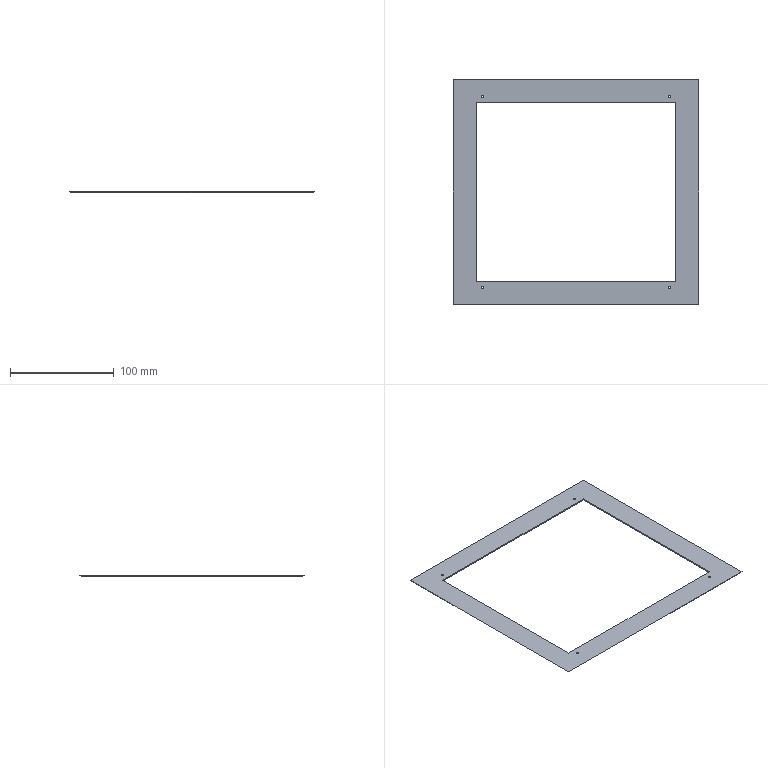Part | NX | 1 solid | 26 faces | box 236.4 x 216.4 x 1.2 mm | volume 21084 mm3 | plane 10 | cone 8 | cylinder 8 | commonest cylinder face diameters 2.5 x8
STEP:
#1=CARTESIAN_POINT('',(-117.,-107.,-75.));
#2=VERTEX_POINT('',#1);
#3=CARTESIAN_POINT('',(-117.,107.,-75.));
#4=VERTEX_POINT('',#3);
#5=CARTESIAN_POINT('',(-117.,0.,-75.));
#6=DIRECTION('',(0.,1.,0.));
#7=VECTOR('',#6,1000.);
#8=LINE('',#5,#7);
#9=EDGE_CURVE('',#2,#4,#8,.T.);
#10=ORIENTED_EDGE('',*,*,#9,.T.);
#11=CARTESIAN_POINT('',(117.,107.,-75.));
#12=VERTEX_POINT('',#11);
#13=CARTESIAN_POINT('',(0.,107.,-75.));
#14=DIRECTION('',(-1.,0.,0.));
#15=VECTOR('',#14,1000.);
#16=LINE('',#13,#15);
#17=EDGE_CURVE('',#12,#4,#16,.T.);
#18=ORIENTED_EDGE('',*,*,#17,.F.);
#19=CARTESIAN_POINT('',(117.,-107.,-75.));
#20=VERTEX_POINT('',#19);
#21=CARTESIAN_POINT('',(117.,0.,-75.));
#22=DIRECTION('',(0.,-1.,0.));
#23=VECTOR('',#22,1000.);
#24=LINE('',#21,#23);
#25=EDGE_CURVE('',#12,#20,#24,.T.);
#26=ORIENTED_EDGE('',*,*,#25,.T.);
#27=CARTESIAN_POINT('',(0.,-107.,-75.));
#28=DIRECTION('',(-1.,0.,0.));
#29=VECTOR('',#28,1000.);
#30=LINE('',#27,#29);
#31=EDGE_CURVE('',#20,#2,#30,.T.);
#32=ORIENTED_EDGE('',*,*,#31,.T.);
#33=EDGE_LOOP('',(#10,#18,#26,#32));
#34=FACE_BOUND('',#33,.T.);
#35=CARTESIAN_POINT('',(-88.3,92.,-75.));
#36=VERTEX_POINT('',#35);
#37=CARTESIAN_POINT('',(-91.7,92.,-75.));
#38=VERTEX_POINT('',#37);
#39=CARTESIAN_POINT('',(-90.,92.,-75.));
#40=DIRECTION('',(0.,0.,-1.));
#41=DIRECTION('',(-1.,0.,0.));
#42=AXIS2_PLACEMENT_3D('',#39,#40,#41);
#43=CIRCLE('',#42,1.7);
#44=EDGE_CURVE('',#36,#38,#43,.T.);
#45=ORIENTED_EDGE('',*,*,#44,.F.);
#46=CARTESIAN_POINT('',(-90.,92.,-75.));
#47=DIRECTION('',(0.,0.,-1.));
#48=DIRECTION('',(-1.,0.,0.));
#49=AXIS2_PLACEMENT_3D('',#46,#47,#48);
#50=CIRCLE('',#49,1.7);
#51=EDGE_CURVE('',#38,#36,#50,.T.);
#52=ORIENTED_EDGE('',*,*,#51,.F.);
#53=EDGE_LOOP('',(#45,#52));
#54=FACE_BOUND('',#53,.T.);
#55=CARTESIAN_POINT('',(91.7,-92.,-75.));
#56=VERTEX_POINT('',#55);
#57=CARTESIAN_POINT('',(88.3,-92.,-75.));
#58=VERTEX_POINT('',#57);
#59=CARTESIAN_POINT('',(90.,-92.,-75.));
#60=DIRECTION('',(0.,0.,-1.));
#61=DIRECTION('',(-1.,0.,0.));
#62=AXIS2_PLACEMENT_3D('',#59,#60,#61);
#63=CIRCLE('',#62,1.7);
#64=EDGE_CURVE('',#56,#58,#63,.T.);
#65=ORIENTED_EDGE('',*,*,#64,.F.);
#66=CARTESIAN_POINT('',(90.,-92.,-75.));
#67=DIRECTION('',(0.,0.,-1.));
#68=DIRECTION('',(-1.,0.,0.));
#69=AXIS2_PLACEMENT_3D('',#66,#67,#68);
#70=CIRCLE('',#69,1.7);
#71=EDGE_CURVE('',#58,#56,#70,.T.);
#72=ORIENTED_EDGE('',*,*,#71,.F.);
#73=EDGE_LOOP('',(#65,#72));
#74=FACE_BOUND('',#73,.T.);
#75=CARTESIAN_POINT('',(-88.3,-92.,-75.));
#76=VERTEX_POINT('',#75);
#77=CARTESIAN_POINT('',(-91.7,-92.,-75.));
#78=VERTEX_POINT('',#77);
#79=CARTESIAN_POINT('',(-90.,-92.,-75.));
#80=DIRECTION('',(0.,0.,-1.));
#81=DIRECTION('',(-1.,0.,0.));
#82=AXIS2_PLACEMENT_3D('',#79,#80,#81);
#83=CIRCLE('',#82,1.7);
#84=EDGE_CURVE('',#76,#78,#83,.T.);
#85=ORIENTED_EDGE('',*,*,#84,.F.);
#86=CARTESIAN_POINT('',(-90.,-92.,-75.));
#87=DIRECTION('',(0.,0.,-1.));
#88=DIRECTION('',(-1.,0.,0.));
#89=AXIS2_PLACEMENT_3D('',#86,#87,#88);
#90=CIRCLE('',#89,1.7);
#91=EDGE_CURVE('',#78,#76,#90,.T.);
#92=ORIENTED_EDGE('',*,*,#91,.F.);
#93=EDGE_LOOP('',(#85,#92));
#94=FACE_BOUND('',#93,.T.);
#95=CARTESIAN_POINT('',(91.7,92.,-75.));
#96=VERTEX_POINT('',#95);
#97=CARTESIAN_POINT('',(88.3,92.,-75.));
#98=VERTEX_POINT('',#97);
#99=CARTESIAN_POINT('',(90.,92.,-75.));
#100=DIRECTION('',(0.,0.,-1.));
#101=DIRECTION('',(-1.,0.,0.));
#102=AXIS2_PLACEMENT_3D('',#99,#100,#101);
#103=CIRCLE('',#102,1.7);
#104=EDGE_CURVE('',#96,#98,#103,.T.);
#105=ORIENTED_EDGE('',*,*,#104,.F.);
#106=CARTESIAN_POINT('',(90.,92.,-75.));
#107=DIRECTION('',(0.,0.,-1.));
#108=DIRECTION('',(-1.,0.,0.));
#109=AXIS2_PLACEMENT_3D('',#106,#107,#108);
#110=CIRCLE('',#109,1.7);
#111=EDGE_CURVE('',#98,#96,#110,.T.);
#112=ORIENTED_EDGE('',*,*,#111,.F.);
#113=EDGE_LOOP('',(#105,#112));
#114=FACE_BOUND('',#113,.T.);
#115=CARTESIAN_POINT('',(-96.,86.,-75.));
#116=VERTEX_POINT('',#115);
#117=CARTESIAN_POINT('',(96.,86.,-75.));
#118=VERTEX_POINT('',#117);
#119=CARTESIAN_POINT('',(0.,86.,-75.));
#120=DIRECTION('',(1.,0.,0.));
#121=VECTOR('',#120,1000.);
#122=LINE('',#119,#121);
#123=EDGE_CURVE('',#116,#118,#122,.T.);
#124=ORIENTED_EDGE('',*,*,#123,.F.);
#125=CARTESIAN_POINT('',(-96.,-86.,-75.));
#126=VERTEX_POINT('',#125);
#127=CARTESIAN_POINT('',(-96.,0.,-75.));
#128=DIRECTION('',(0.,1.,0.));
#129=VECTOR('',#128,1000.);
#130=LINE('',#127,#129);
#131=EDGE_CURVE('',#126,#116,#130,.T.);
#132=ORIENTED_EDGE('',*,*,#131,.F.);
#133=CARTESIAN_POINT('',(96.,-86.,-75.));
#134=VERTEX_POINT('',#133);
#135=CARTESIAN_POINT('',(0.,-86.,-75.));
#136=DIRECTION('',(-1.,0.,0.));
#137=VECTOR('',#136,1000.);
#138=LINE('',#135,#137);
#139=EDGE_CURVE('',#134,#126,#138,.T.);
#140=ORIENTED_EDGE('',*,*,#139,.F.);
#141=CARTESIAN_POINT('',(96.,0.,-75.));
#142=DIRECTION('',(0.,-1.,0.));
#143=VECTOR('',#142,1000.);
#144=LINE('',#141,#143);
#145=EDGE_CURVE('',#118,#134,#144,.T.);
#146=ORIENTED_EDGE('',*,*,#145,.F.);
#147=EDGE_LOOP('',(#124,#132,#140,#146));
#148=FACE_BOUND('',#147,.T.);
#149=CARTESIAN_POINT('',(0.,0.,-75.));
#150=DIRECTION('',(0.,0.,1.));
#151=DIRECTION('',(1.,0.,0.));
#152=AXIS2_PLACEMENT_3D('',#149,#150,#151);
#153=PLANE('',#152);
#154=ADVANCED_FACE('',(#34,#54,#74,#94,#114,#148),#153,.F.);
#155=CARTESIAN_POINT('',(-88.75,92.,-74.74));
#156=VERTEX_POINT('',#155);
#157=CARTESIAN_POINT('',(-91.25,92.,-74.74));
#158=VERTEX_POINT('',#157);
#159=CARTESIAN_POINT('',(-90.,92.,-74.74));
#160=DIRECTION('',(0.,0.,-1.));
#161=DIRECTION('',(-1.,0.,0.));
#162=AXIS2_PLACEMENT_3D('',#159,#160,#161);
#163=CIRCLE('',#162,1.25);
#164=EDGE_CURVE('',#156,#158,#163,.T.);
#165=ORIENTED_EDGE('',*,*,#164,.F.);
#166=CARTESIAN_POINT('',(-88.75,92.,-74.74));
#167=DIRECTION('',(0.866,0.,-0.5));
#168=VECTOR('',#167,1000.);
#169=LINE('',#166,#168);
#170=EDGE_CURVE('',#36,#156,#169,.F.);
#171=ORIENTED_EDGE('',*,*,#170,.F.);
#172=ORIENTED_EDGE('',*,*,#44,.T.);
#173=CARTESIAN_POINT('',(-91.25,92.,-74.74));
#174=DIRECTION('',(-0.866,0.,-0.5));
#175=VECTOR('',#174,1000.);
#176=LINE('',#173,#175);
#177=EDGE_CURVE('',#38,#158,#176,.F.);
#178=ORIENTED_EDGE('',*,*,#177,.T.);
#179=EDGE_LOOP('',(#165,#171,#172,#178));
#180=FACE_BOUND('',#179,.T.);
#181=CARTESIAN_POINT('',(-90.,92.,-74.74));
#182=DIRECTION('',(0.,0.,-1.));
#183=DIRECTION('',(-1.,0.,0.));
#184=AXIS2_PLACEMENT_3D('',#181,#182,#183);
#185=CONICAL_SURFACE('',#184,1.25,1.047);
#186=ADVANCED_FACE('',(#180),#185,.F.);
#187=ORIENTED_EDGE('',*,*,#164,.T.);
#188=CARTESIAN_POINT('',(-91.25,92.,-73.8));
#189=VERTEX_POINT('',#188);
#190=CARTESIAN_POINT('',(-91.25,92.,-75.));
#191=DIRECTION('',(0.,0.,-1.));
#192=VECTOR('',#191,1000.);
#193=LINE('',#190,#192);
#194=EDGE_CURVE('',#158,#189,#193,.F.);
#195=ORIENTED_EDGE('',*,*,#194,.T.);
#196=CARTESIAN_POINT('',(-88.75,92.,-73.8));
#197=VERTEX_POINT('',#196);
#198=CARTESIAN_POINT('',(-90.,92.,-73.8));
#199=DIRECTION('',(0.,0.,-1.));
#200=DIRECTION('',(-1.,0.,0.));
#201=AXIS2_PLACEMENT_3D('',#198,#199,#200);
#202=CIRCLE('',#201,1.25);
#203=EDGE_CURVE('',#197,#189,#202,.T.);
#204=ORIENTED_EDGE('',*,*,#203,.F.);
#205=CARTESIAN_POINT('',(-88.75,92.,-75.));
#206=DIRECTION('',(0.,0.,-1.));
#207=VECTOR('',#206,1000.);
#208=LINE('',#205,#207);
#209=EDGE_CURVE('',#156,#197,#208,.F.);
#210=ORIENTED_EDGE('',*,*,#209,.F.);
#211=EDGE_LOOP('',(#187,#195,#204,#210));
#212=FACE_BOUND('',#211,.T.);
#213=CARTESIAN_POINT('',(-90.,92.,-75.));
#214=DIRECTION('',(0.,0.,-1.));
#215=DIRECTION('',(-1.,0.,0.));
#216=AXIS2_PLACEMENT_3D('',#213,#214,#215);
#217=CYLINDRICAL_SURFACE('',#216,1.25);
#218=ADVANCED_FACE('',(#212),#217,.F.);
#219=CARTESIAN_POINT('',(118.2,108.2,-73.8));
#220=VERTEX_POINT('',#219);
#221=CARTESIAN_POINT('',(118.2,-108.2,-73.8));
#222=VERTEX_POINT('',#221);
#223=CARTESIAN_POINT('',(118.2,0.,-73.8));
#224=DIRECTION('',(0.,-1.,0.));
#225=VECTOR('',#224,1000.);
#226=LINE('',#223,#225);
#227=EDGE_CURVE('',#220,#222,#226,.T.);
#228=ORIENTED_EDGE('',*,*,#227,.F.);
#229=CARTESIAN_POINT('',(-118.2,108.2,-73.8));
#230=VERTEX_POINT('',#229);
#231=CARTESIAN_POINT('',(0.,108.2,-73.8));
#232=DIRECTION('',(1.,0.,0.));
#233=VECTOR('',#232,1000.);
#234=LINE('',#231,#233);
#235=EDGE_CURVE('',#230,#220,#234,.T.);
#236=ORIENTED_EDGE('',*,*,#235,.F.);
#237=CARTESIAN_POINT('',(-118.2,-108.2,-73.8));
#238=VERTEX_POINT('',#237);
#239=CARTESIAN_POINT('',(-118.2,0.,-73.8));
#240=DIRECTION('',(0.,1.,0.));
#241=VECTOR('',#240,1000.);
#242=LINE('',#239,#241);
#243=EDGE_CURVE('',#238,#230,#242,.T.);
#244=ORIENTED_EDGE('',*,*,#243,.F.);
#245=CARTESIAN_POINT('',(0.,-108.2,-73.8));
#246=DIRECTION('',(1.,0.,0.));
#247=VECTOR('',#246,1000.);
#248=LINE('',#245,#247);
#249=EDGE_CURVE('',#238,#222,#248,.T.);
#250=ORIENTED_EDGE('',*,*,#249,.T.);
#251=EDGE_LOOP('',(#228,#236,#244,#250));
#252=FACE_BOUND('',#251,.T.);
#253=CARTESIAN_POINT('',(96.,86.,-73.8));
#254=VERTEX_POINT('',#253);
#255=CARTESIAN_POINT('',(-96.,86.,-73.8));
#256=VERTEX_POINT('',#255);
#257=CARTESIAN_POINT('',(0.,86.,-73.8));
#258=DIRECTION('',(-1.,0.,0.));
#259=VECTOR('',#258,1000.);
#260=LINE('',#257,#259);
#261=EDGE_CURVE('',#254,#256,#260,.T.);
#262=ORIENTED_EDGE('',*,*,#261,.F.);
#263=CARTESIAN_POINT('',(96.,-86.,-73.8));
#264=VERTEX_POINT('',#263);
#265=CARTESIAN_POINT('',(96.,0.,-73.8));
#266=DIRECTION('',(0.,1.,0.));
#267=VECTOR('',#266,1000.);
#268=LINE('',#265,#267);
#269=EDGE_CURVE('',#264,#254,#268,.T.);
#270=ORIENTED_EDGE('',*,*,#269,.F.);
#271=CARTESIAN_POINT('',(-96.,-86.,-73.8));
#272=VERTEX_POINT('',#271);
#273=CARTESIAN_POINT('',(0.,-86.,-73.8));
#274=DIRECTION('',(1.,0.,0.));
#275=VECTOR('',#274,1000.);
#276=LINE('',#273,#275);
#277=EDGE_CURVE('',#272,#264,#276,.T.);
#278=ORIENTED_EDGE('',*,*,#277,.F.);
#279=CARTESIAN_POINT('',(-96.,0.,-73.8));
#280=DIRECTION('',(0.,-1.,0.));
#281=VECTOR('',#280,1000.);
#282=LINE('',#279,#281);
#283=EDGE_CURVE('',#256,#272,#282,.T.);
#284=ORIENTED_EDGE('',*,*,#283,.F.);
#285=EDGE_LOOP('',(#262,#270,#278,#284));
#286=FACE_BOUND('',#285,.T.);
#287=CARTESIAN_POINT('',(-88.75,-92.,-73.8));
#288=VERTEX_POINT('',#287);
#289=CARTESIAN_POINT('',(-91.25,-92.,-73.8));
#290=VERTEX_POINT('',#289);
#291=CARTESIAN_POINT('',(-90.,-92.,-73.8));
#292=DIRECTION('',(0.,0.,-1.));
#293=DIRECTION('',(-1.,0.,0.));
#294=AXIS2_PLACEMENT_3D('',#291,#292,#293);
#295=CIRCLE('',#294,1.25);
#296=EDGE_CURVE('',#288,#290,#295,.T.);
#297=ORIENTED_EDGE('',*,*,#296,.T.);
#298=CARTESIAN_POINT('',(-90.,-92.,-73.8));
#299=DIRECTION('',(0.,0.,-1.));
#300=DIRECTION('',(-1.,0.,0.));
#301=AXIS2_PLACEMENT_3D('',#298,#299,#300);
#302=CIRCLE('',#301,1.25);
#303=EDGE_CURVE('',#290,#288,#302,.T.);
#304=ORIENTED_EDGE('',*,*,#303,.T.);
#305=EDGE_LOOP('',(#297,#304));
#306=FACE_BOUND('',#305,.T.);
#307=CARTESIAN_POINT('',(91.25,-92.,-73.8));
#308=VERTEX_POINT('',#307);
#309=CARTESIAN_POINT('',(88.75,-92.,-73.8));
#310=VERTEX_POINT('',#309);
#311=CARTESIAN_POINT('',(90.,-92.,-73.8));
#312=DIRECTION('',(0.,0.,-1.));
#313=DIRECTION('',(-1.,0.,0.));
#314=AXIS2_PLACEMENT_3D('',#311,#312,#313);
#315=CIRCLE('',#314,1.25);
#316=EDGE_CURVE('',#308,#310,#315,.T.);
#317=ORIENTED_EDGE('',*,*,#316,.T.);
#318=CARTESIAN_POINT('',(90.,-92.,-73.8));
#319=DIRECTION('',(0.,0.,-1.));
#320=DIRECTION('',(-1.,0.,0.));
#321=AXIS2_PLACEMENT_3D('',#318,#319,#320);
#322=CIRCLE('',#321,1.25);
#323=EDGE_CURVE('',#310,#308,#322,.T.);
#324=ORIENTED_EDGE('',*,*,#323,.T.);
#325=EDGE_LOOP('',(#317,#324));
#326=FACE_BOUND('',#325,.T.);
#327=CARTESIAN_POINT('',(91.25,92.,-73.8));
#328=VERTEX_POINT('',#327);
#329=CARTESIAN_POINT('',(88.75,92.,-73.8));
#330=VERTEX_POINT('',#329);
#331=CARTESIAN_POINT('',(90.,92.,-73.8));
#332=DIRECTION('',(0.,0.,-1.));
#333=DIRECTION('',(-1.,0.,0.));
#334=AXIS2_PLACEMENT_3D('',#331,#332,#333);
#335=CIRCLE('',#334,1.25);
#336=EDGE_CURVE('',#328,#330,#335,.T.);
#337=ORIENTED_EDGE('',*,*,#336,.T.);
#338=CARTESIAN_POINT('',(90.,92.,-73.8));
#339=DIRECTION('',(0.,0.,-1.));
#340=DIRECTION('',(-1.,0.,0.));
#341=AXIS2_PLACEMENT_3D('',#338,#339,#340);
#342=CIRCLE('',#341,1.25);
#343=EDGE_CURVE('',#330,#328,#342,.T.);
#344=ORIENTED_EDGE('',*,*,#343,.T.);
#345=EDGE_LOOP('',(#337,#344));
#346=FACE_BOUND('',#345,.T.);
#347=ORIENTED_EDGE('',*,*,#203,.T.);
#348=CARTESIAN_POINT('',(-90.,92.,-73.8));
#349=DIRECTION('',(0.,0.,-1.));
#350=DIRECTION('',(-1.,0.,0.));
#351=AXIS2_PLACEMENT_3D('',#348,#349,#350);
#352=CIRCLE('',#351,1.25);
#353=EDGE_CURVE('',#189,#197,#352,.T.);
#354=ORIENTED_EDGE('',*,*,#353,.T.);
#355=EDGE_LOOP('',(#347,#354));
#356=FACE_BOUND('',#355,.T.);
#357=CARTESIAN_POINT('',(0.,0.,-73.8));
#358=DIRECTION('',(0.,0.,-1.));
#359=DIRECTION('',(0.,-1.,0.));
#360=AXIS2_PLACEMENT_3D('',#357,#358,#359);
#361=PLANE('',#360);
#362=ADVANCED_FACE('',(#252,#286,#306,#326,#346,#356),#361,.F.);
#363=ORIENTED_EDGE('',*,*,#9,.F.);
#364=CARTESIAN_POINT('',(-192.,-182.,0.));
#365=DIRECTION('',(0.5774,0.5774,-0.5774));
#366=VECTOR('',#365,1000.);
#367=LINE('',#364,#366);
#368=EDGE_CURVE('',#238,#2,#367,.T.);
#369=ORIENTED_EDGE('',*,*,#368,.F.);
#370=ORIENTED_EDGE('',*,*,#243,.T.);
#371=CARTESIAN_POINT('',(-192.,182.,0.));
#372=DIRECTION('',(0.5774,-0.5774,-0.5774));
#373=VECTOR('',#372,1000.);
#374=LINE('',#371,#373);
#375=EDGE_CURVE('',#230,#4,#374,.T.);
#376=ORIENTED_EDGE('',*,*,#375,.T.);
#377=EDGE_LOOP('',(#363,#369,#370,#376));
#378=FACE_BOUND('',#377,.T.);
#379=CARTESIAN_POINT('',(-118.5,0.,-73.5));
#380=DIRECTION('',(-0.7071,0.,-0.7071));
#381=DIRECTION('',(-0.7071,0.,0.7071));
#382=AXIS2_PLACEMENT_3D('',#379,#380,#381);
#383=PLANE('',#382);
#384=ADVANCED_FACE('',(#378),#383,.T.);
#385=ORIENTED_EDGE('',*,*,#25,.F.);
#386=CARTESIAN_POINT('',(192.,182.,0.));
#387=DIRECTION('',(-0.5774,-0.5774,-0.5774));
#388=VECTOR('',#387,1000.);
#389=LINE('',#386,#388);
#390=EDGE_CURVE('',#220,#12,#389,.T.);
#391=ORIENTED_EDGE('',*,*,#390,.F.);
#392=ORIENTED_EDGE('',*,*,#227,.T.);
#393=CARTESIAN_POINT('',(192.,-182.,0.));
#394=DIRECTION('',(-0.5774,0.5774,-0.5774));
#395=VECTOR('',#394,1000.);
#396=LINE('',#393,#395);
#397=EDGE_CURVE('',#222,#20,#396,.T.);
#398=ORIENTED_EDGE('',*,*,#397,.T.);
#399=EDGE_LOOP('',(#385,#391,#392,#398));
#400=FACE_BOUND('',#399,.T.);
#401=CARTESIAN_POINT('',(118.5,0.,-73.5));
#402=DIRECTION('',(0.7071,0.,-0.7071));
#403=DIRECTION('',(0.,-1.,0.));
#404=AXIS2_PLACEMENT_3D('',#401,#402,#403);
#405=PLANE('',#404);
#406=ADVANCED_FACE('',(#400),#405,.T.);
#407=ORIENTED_EDGE('',*,*,#235,.T.);
#408=ORIENTED_EDGE('',*,*,#390,.T.);
#409=ORIENTED_EDGE('',*,*,#17,.T.);
#410=ORIENTED_EDGE('',*,*,#375,.F.);
#411=EDGE_LOOP('',(#407,#408,#409,#410));
#412=FACE_BOUND('',#411,.T.);
#413=CARTESIAN_POINT('',(0.,108.5,-73.5));
#414=DIRECTION('',(0.,0.7071,-0.7071));
#415=DIRECTION('',(-1.,0.,0.));
#416=AXIS2_PLACEMENT_3D('',#413,#414,#415);
#417=PLANE('',#416);
#418=ADVANCED_FACE('',(#412),#417,.T.);
#419=ORIENTED_EDGE('',*,*,#249,.F.);
#420=ORIENTED_EDGE('',*,*,#368,.T.);
#421=ORIENTED_EDGE('',*,*,#31,.F.);
#422=ORIENTED_EDGE('',*,*,#397,.F.);
#423=EDGE_LOOP('',(#419,#420,#421,#422));
#424=FACE_BOUND('',#423,.T.);
#425=CARTESIAN_POINT('',(0.,-108.5,-73.5));
#426=DIRECTION('',(0.,0.7071,0.7071));
#427=DIRECTION('',(1.,0.,0.));
#428=AXIS2_PLACEMENT_3D('',#425,#426,#427);
#429=PLANE('',#428);
#430=ADVANCED_FACE('',(#424),#429,.F.);
#431=ORIENTED_EDGE('',*,*,#261,.T.);
#432=CARTESIAN_POINT('',(-96.,86.,-73.8));
#433=DIRECTION('',(0.,0.,-1.));
#434=VECTOR('',#433,1000.);
#435=LINE('',#432,#434);
#436=EDGE_CURVE('',#256,#116,#435,.T.);
#437=ORIENTED_EDGE('',*,*,#436,.T.);
#438=ORIENTED_EDGE('',*,*,#123,.T.);
#439=CARTESIAN_POINT('',(96.,86.,-73.8));
#440=DIRECTION('',(0.,0.,-1.));
#441=VECTOR('',#440,1000.);
#442=LINE('',#439,#441);
#443=EDGE_CURVE('',#254,#118,#442,.T.);
#444=ORIENTED_EDGE('',*,*,#443,.F.);
#445=EDGE_LOOP('',(#431,#437,#438,#444));
#446=FACE_BOUND('',#445,.T.);
#447=CARTESIAN_POINT('',(-96.,86.,-75.));
#448=DIRECTION('',(0.,1.,0.));
#449=DIRECTION('',(1.,0.,0.));
#450=AXIS2_PLACEMENT_3D('',#447,#448,#449);
#451=PLANE('',#450);
#452=ADVANCED_FACE('',(#446),#451,.F.);
#453=ORIENTED_EDGE('',*,*,#277,.T.);
#454=CARTESIAN_POINT('',(96.,-86.,-73.8));
#455=DIRECTION('',(0.,0.,-1.));
#456=VECTOR('',#455,1000.);
#457=LINE('',#454,#456);
#458=EDGE_CURVE('',#264,#134,#457,.T.);
#459=ORIENTED_EDGE('',*,*,#458,.T.);
#460=ORIENTED_EDGE('',*,*,#139,.T.);
#461=CARTESIAN_POINT('',(-96.,-86.,-73.8));
#462=DIRECTION('',(0.,0.,-1.));
#463=VECTOR('',#462,1000.);
#464=LINE('',#461,#463);
#465=EDGE_CURVE('',#272,#126,#464,.T.);
#466=ORIENTED_EDGE('',*,*,#465,.F.);
#467=EDGE_LOOP('',(#453,#459,#460,#466));
#468=FACE_BOUND('',#467,.T.);
#469=CARTESIAN_POINT('',(96.,-86.,-75.));
#470=DIRECTION('',(0.,-1.,0.));
#471=DIRECTION('',(0.,0.,-1.));
#472=AXIS2_PLACEMENT_3D('',#469,#470,#471);
#473=PLANE('',#472);
#474=ADVANCED_FACE('',(#468),#473,.F.);
#475=ORIENTED_EDGE('',*,*,#283,.T.);
#476=ORIENTED_EDGE('',*,*,#465,.T.);
#477=ORIENTED_EDGE('',*,*,#131,.T.);
#478=ORIENTED_EDGE('',*,*,#436,.F.);
#479=EDGE_LOOP('',(#475,#476,#477,#478));
#480=FACE_BOUND('',#479,.T.);
#481=CARTESIAN_POINT('',(-96.,-86.,-75.));
#482=DIRECTION('',(-1.,0.,0.));
#483=DIRECTION('',(0.,0.,1.));
#484=AXIS2_PLACEMENT_3D('',#481,#482,#483);
#485=PLANE('',#484);
#486=ADVANCED_FACE('',(#480),#485,.F.);
#487=ORIENTED_EDGE('',*,*,#269,.T.);
#488=ORIENTED_EDGE('',*,*,#443,.T.);
#489=ORIENTED_EDGE('',*,*,#145,.T.);
#490=ORIENTED_EDGE('',*,*,#458,.F.);
#491=EDGE_LOOP('',(#487,#488,#489,#490));
#492=FACE_BOUND('',#491,.T.);
#493=CARTESIAN_POINT('',(96.,86.,-75.));
#494=DIRECTION('',(1.,0.,0.));
#495=DIRECTION('',(0.,1.,0.));
#496=AXIS2_PLACEMENT_3D('',#493,#494,#495);
#497=PLANE('',#496);
#498=ADVANCED_FACE('',(#492),#497,.F.);
#499=CARTESIAN_POINT('',(-88.75,-92.,-74.74));
#500=VERTEX_POINT('',#499);
#501=CARTESIAN_POINT('',(-91.25,-92.,-74.74));
#502=VERTEX_POINT('',#501);
#503=CARTESIAN_POINT('',(-90.,-92.,-74.74));
#504=DIRECTION('',(0.,0.,-1.));
#505=DIRECTION('',(-1.,0.,0.));
#506=AXIS2_PLACEMENT_3D('',#503,#504,#505);
#507=CIRCLE('',#506,1.25);
#508=EDGE_CURVE('',#500,#502,#507,.T.);
#509=ORIENTED_EDGE('',*,*,#508,.T.);
#510=CARTESIAN_POINT('',(-91.25,-92.,-75.));
#511=DIRECTION('',(0.,0.,-1.));
#512=VECTOR('',#511,1000.);
#513=LINE('',#510,#512);
#514=EDGE_CURVE('',#502,#290,#513,.F.);
#515=ORIENTED_EDGE('',*,*,#514,.T.);
#516=ORIENTED_EDGE('',*,*,#296,.F.);
#517=CARTESIAN_POINT('',(-88.75,-92.,-75.));
#518=DIRECTION('',(0.,0.,-1.));
#519=VECTOR('',#518,1000.);
#520=LINE('',#517,#519);
#521=EDGE_CURVE('',#500,#288,#520,.F.);
#522=ORIENTED_EDGE('',*,*,#521,.F.);
#523=EDGE_LOOP('',(#509,#515,#516,#522));
#524=FACE_BOUND('',#523,.T.);
#525=CARTESIAN_POINT('',(-90.,-92.,-75.));
#526=DIRECTION('',(0.,0.,-1.));
#527=DIRECTION('',(-1.,0.,0.));
#528=AXIS2_PLACEMENT_3D('',#525,#526,#527);
#529=CYLINDRICAL_SURFACE('',#528,1.25);
#530=ADVANCED_FACE('',(#524),#529,.F.);
#531=ORIENTED_EDGE('',*,*,#508,.F.);
#532=CARTESIAN_POINT('',(-88.75,-92.,-74.74));
#533=DIRECTION('',(0.866,0.,-0.5));
#534=VECTOR('',#533,1000.);
#535=LINE('',#532,#534);
#536=EDGE_CURVE('',#76,#500,#535,.F.);
#537=ORIENTED_EDGE('',*,*,#536,.F.);
#538=ORIENTED_EDGE('',*,*,#84,.T.);
#539=CARTESIAN_POINT('',(-91.25,-92.,-74.74));
#540=DIRECTION('',(-0.866,0.,-0.5));
#541=VECTOR('',#540,1000.);
#542=LINE('',#539,#541);
#543=EDGE_CURVE('',#78,#502,#542,.F.);
#544=ORIENTED_EDGE('',*,*,#543,.T.);
#545=EDGE_LOOP('',(#531,#537,#538,#544));
#546=FACE_BOUND('',#545,.T.);
#547=CARTESIAN_POINT('',(-90.,-92.,-74.74));
#548=DIRECTION('',(0.,0.,-1.));
#549=DIRECTION('',(-1.,0.,0.));
#550=AXIS2_PLACEMENT_3D('',#547,#548,#549);
#551=CONICAL_SURFACE('',#550,1.25,1.047);
#552=ADVANCED_FACE('',(#546),#551,.F.);
#553=CARTESIAN_POINT('',(91.25,-92.,-74.74));
#554=VERTEX_POINT('',#553);
#555=CARTESIAN_POINT('',(88.75,-92.,-74.74));
#556=VERTEX_POINT('',#555);
#557=CARTESIAN_POINT('',(90.,-92.,-74.74));
#558=DIRECTION('',(0.,0.,-1.));
#559=DIRECTION('',(-1.,0.,0.));
#560=AXIS2_PLACEMENT_3D('',#557,#558,#559);
#561=CIRCLE('',#560,1.25);
#562=EDGE_CURVE('',#554,#556,#561,.T.);
#563=ORIENTED_EDGE('',*,*,#562,.T.);
#564=CARTESIAN_POINT('',(88.75,-92.,-75.));
#565=DIRECTION('',(0.,0.,-1.));
#566=VECTOR('',#565,1000.);
#567=LINE('',#564,#566);
#568=EDGE_CURVE('',#556,#310,#567,.F.);
#569=ORIENTED_EDGE('',*,*,#568,.T.);
#570=ORIENTED_EDGE('',*,*,#316,.F.);
#571=CARTESIAN_POINT('',(91.25,-92.,-75.));
#572=DIRECTION('',(0.,0.,-1.));
#573=VECTOR('',#572,1000.);
#574=LINE('',#571,#573);
#575=EDGE_CURVE('',#554,#308,#574,.F.);
#576=ORIENTED_EDGE('',*,*,#575,.F.);
#577=EDGE_LOOP('',(#563,#569,#570,#576));
#578=FACE_BOUND('',#577,.T.);
#579=CARTESIAN_POINT('',(90.,-92.,-75.));
#580=DIRECTION('',(0.,0.,-1.));
#581=DIRECTION('',(-1.,0.,0.));
#582=AXIS2_PLACEMENT_3D('',#579,#580,#581);
#583=CYLINDRICAL_SURFACE('',#582,1.25);
#584=ADVANCED_FACE('',(#578),#583,.F.);
#585=ORIENTED_EDGE('',*,*,#562,.F.);
#586=CARTESIAN_POINT('',(91.25,-92.,-74.74));
#587=DIRECTION('',(0.866,0.,-0.5));
#588=VECTOR('',#587,1000.);
#589=LINE('',#586,#588);
#590=EDGE_CURVE('',#56,#554,#589,.F.);
#591=ORIENTED_EDGE('',*,*,#590,.F.);
#592=ORIENTED_EDGE('',*,*,#64,.T.);
#593=CARTESIAN_POINT('',(88.75,-92.,-74.74));
#594=DIRECTION('',(-0.866,0.,-0.5));
#595=VECTOR('',#594,1000.);
#596=LINE('',#593,#595);
#597=EDGE_CURVE('',#58,#556,#596,.F.);
#598=ORIENTED_EDGE('',*,*,#597,.T.);
#599=EDGE_LOOP('',(#585,#591,#592,#598));
#600=FACE_BOUND('',#599,.T.);
#601=CARTESIAN_POINT('',(90.,-92.,-74.74));
#602=DIRECTION('',(0.,0.,-1.));
#603=DIRECTION('',(-1.,0.,0.));
#604=AXIS2_PLACEMENT_3D('',#601,#602,#603);
#605=CONICAL_SURFACE('',#604,1.25,1.047);
#606=ADVANCED_FACE('',(#600),#605,.F.);
#607=CARTESIAN_POINT('',(91.25,92.,-74.74));
#608=VERTEX_POINT('',#607);
#609=CARTESIAN_POINT('',(88.75,92.,-74.74));
#610=VERTEX_POINT('',#609);
#611=CARTESIAN_POINT('',(90.,92.,-74.74));
#612=DIRECTION('',(0.,0.,-1.));
#613=DIRECTION('',(-1.,0.,0.));
#614=AXIS2_PLACEMENT_3D('',#611,#612,#613);
#615=CIRCLE('',#614,1.25);
#616=EDGE_CURVE('',#608,#610,#615,.T.);
#617=ORIENTED_EDGE('',*,*,#616,.T.);
#618=CARTESIAN_POINT('',(88.75,92.,-75.));
#619=DIRECTION('',(0.,0.,-1.));
#620=VECTOR('',#619,1000.);
#621=LINE('',#618,#620);
#622=EDGE_CURVE('',#610,#330,#621,.F.);
#623=ORIENTED_EDGE('',*,*,#622,.T.);
#624=ORIENTED_EDGE('',*,*,#336,.F.);
#625=CARTESIAN_POINT('',(91.25,92.,-75.));
#626=DIRECTION('',(0.,0.,-1.));
#627=VECTOR('',#626,1000.);
#628=LINE('',#625,#627);
#629=EDGE_CURVE('',#608,#328,#628,.F.);
#630=ORIENTED_EDGE('',*,*,#629,.F.);
#631=EDGE_LOOP('',(#617,#623,#624,#630));
#632=FACE_BOUND('',#631,.T.);
#633=CARTESIAN_POINT('',(90.,92.,-75.));
#634=DIRECTION('',(0.,0.,-1.));
#635=DIRECTION('',(-1.,0.,0.));
#636=AXIS2_PLACEMENT_3D('',#633,#634,#635);
#637=CYLINDRICAL_SURFACE('',#636,1.25);
#638=ADVANCED_FACE('',(#632),#637,.F.);
#639=ORIENTED_EDGE('',*,*,#616,.F.);
#640=CARTESIAN_POINT('',(91.25,92.,-74.74));
#641=DIRECTION('',(0.866,0.,-0.5));
#642=VECTOR('',#641,1000.);
#643=LINE('',#640,#642);
#644=EDGE_CURVE('',#96,#608,#643,.F.);
#645=ORIENTED_EDGE('',*,*,#644,.F.);
#646=ORIENTED_EDGE('',*,*,#104,.T.);
#647=CARTESIAN_POINT('',(88.75,92.,-74.74));
#648=DIRECTION('',(-0.866,0.,-0.5));
#649=VECTOR('',#648,1000.);
#650=LINE('',#647,#649);
#651=EDGE_CURVE('',#98,#610,#650,.F.);
#652=ORIENTED_EDGE('',*,*,#651,.T.);
#653=EDGE_LOOP('',(#639,#645,#646,#652));
#654=FACE_BOUND('',#653,.T.);
#655=CARTESIAN_POINT('',(90.,92.,-74.74));
#656=DIRECTION('',(0.,0.,-1.));
#657=DIRECTION('',(-1.,0.,0.));
#658=AXIS2_PLACEMENT_3D('',#655,#656,#657);
#659=CONICAL_SURFACE('',#658,1.25,1.047);
#660=ADVANCED_FACE('',(#654),#659,.F.);
#661=ORIENTED_EDGE('',*,*,#568,.F.);
#662=CARTESIAN_POINT('',(90.,-92.,-74.74));
#663=DIRECTION('',(0.,0.,-1.));
#664=DIRECTION('',(-1.,0.,0.));
#665=AXIS2_PLACEMENT_3D('',#662,#663,#664);
#666=CIRCLE('',#665,1.25);
#667=EDGE_CURVE('',#556,#554,#666,.T.);
#668=ORIENTED_EDGE('',*,*,#667,.T.);
#669=ORIENTED_EDGE('',*,*,#575,.T.);
#670=ORIENTED_EDGE('',*,*,#323,.F.);
#671=EDGE_LOOP('',(#661,#668,#669,#670));
#672=FACE_BOUND('',#671,.T.);
#673=CARTESIAN_POINT('',(90.,-92.,-75.));
#674=DIRECTION('',(0.,0.,-1.));
#675=DIRECTION('',(-1.,0.,0.));
#676=AXIS2_PLACEMENT_3D('',#673,#674,#675);
#677=CYLINDRICAL_SURFACE('',#676,1.25);
#678=ADVANCED_FACE('',(#672),#677,.F.);
#679=ORIENTED_EDGE('',*,*,#597,.F.);
#680=ORIENTED_EDGE('',*,*,#71,.T.);
#681=ORIENTED_EDGE('',*,*,#590,.T.);
#682=ORIENTED_EDGE('',*,*,#667,.F.);
#683=EDGE_LOOP('',(#679,#680,#681,#682));
#684=FACE_BOUND('',#683,.T.);
#685=CARTESIAN_POINT('',(90.,-92.,-74.74));
#686=DIRECTION('',(0.,0.,-1.));
#687=DIRECTION('',(-1.,0.,0.));
#688=AXIS2_PLACEMENT_3D('',#685,#686,#687);
#689=CONICAL_SURFACE('',#688,1.25,1.047);
#690=ADVANCED_FACE('',(#684),#689,.F.);
#691=ORIENTED_EDGE('',*,*,#651,.F.);
#692=ORIENTED_EDGE('',*,*,#111,.T.);
#693=ORIENTED_EDGE('',*,*,#644,.T.);
#694=CARTESIAN_POINT('',(90.,92.,-74.74));
#695=DIRECTION('',(0.,0.,-1.));
#696=DIRECTION('',(-1.,0.,0.));
#697=AXIS2_PLACEMENT_3D('',#694,#695,#696);
#698=CIRCLE('',#697,1.25);
#699=EDGE_CURVE('',#610,#608,#698,.T.);
#700=ORIENTED_EDGE('',*,*,#699,.F.);
#701=EDGE_LOOP('',(#691,#692,#693,#700));
#702=FACE_BOUND('',#701,.T.);
#703=CARTESIAN_POINT('',(90.,92.,-74.74));
#704=DIRECTION('',(0.,0.,-1.));
#705=DIRECTION('',(-1.,0.,0.));
#706=AXIS2_PLACEMENT_3D('',#703,#704,#705);
#707=CONICAL_SURFACE('',#706,1.25,1.047);
#708=ADVANCED_FACE('',(#702),#707,.F.);
#709=ORIENTED_EDGE('',*,*,#622,.F.);
#710=ORIENTED_EDGE('',*,*,#699,.T.);
#711=ORIENTED_EDGE('',*,*,#629,.T.);
#712=ORIENTED_EDGE('',*,*,#343,.F.);
#713=EDGE_LOOP('',(#709,#710,#711,#712));
#714=FACE_BOUND('',#713,.T.);
#715=CARTESIAN_POINT('',(90.,92.,-75.));
#716=DIRECTION('',(0.,0.,-1.));
#717=DIRECTION('',(-1.,0.,0.));
#718=AXIS2_PLACEMENT_3D('',#715,#716,#717);
#719=CYLINDRICAL_SURFACE('',#718,1.25);
#720=ADVANCED_FACE('',(#714),#719,.F.);
#721=ORIENTED_EDGE('',*,*,#514,.F.);
#722=CARTESIAN_POINT('',(-90.,-92.,-74.74));
#723=DIRECTION('',(0.,0.,-1.));
#724=DIRECTION('',(-1.,0.,0.));
#725=AXIS2_PLACEMENT_3D('',#722,#723,#724);
#726=CIRCLE('',#725,1.25);
#727=EDGE_CURVE('',#502,#500,#726,.T.);
#728=ORIENTED_EDGE('',*,*,#727,.T.);
#729=ORIENTED_EDGE('',*,*,#521,.T.);
#730=ORIENTED_EDGE('',*,*,#303,.F.);
#731=EDGE_LOOP('',(#721,#728,#729,#730));
#732=FACE_BOUND('',#731,.T.);
#733=CARTESIAN_POINT('',(-90.,-92.,-75.));
#734=DIRECTION('',(0.,0.,-1.));
#735=DIRECTION('',(-1.,0.,0.));
#736=AXIS2_PLACEMENT_3D('',#733,#734,#735);
#737=CYLINDRICAL_SURFACE('',#736,1.25);
#738=ADVANCED_FACE('',(#732),#737,.F.);
#739=ORIENTED_EDGE('',*,*,#194,.F.);
#740=CARTESIAN_POINT('',(-90.,92.,-74.74));
#741=DIRECTION('',(0.,0.,-1.));
#742=DIRECTION('',(-1.,0.,0.));
#743=AXIS2_PLACEMENT_3D('',#740,#741,#742);
#744=CIRCLE('',#743,1.25);
#745=EDGE_CURVE('',#158,#156,#744,.T.);
#746=ORIENTED_EDGE('',*,*,#745,.T.);
#747=ORIENTED_EDGE('',*,*,#209,.T.);
#748=ORIENTED_EDGE('',*,*,#353,.F.);
#749=EDGE_LOOP('',(#739,#746,#747,#748));
#750=FACE_BOUND('',#749,.T.);
#751=CARTESIAN_POINT('',(-90.,92.,-75.));
#752=DIRECTION('',(0.,0.,-1.));
#753=DIRECTION('',(-1.,0.,0.));
#754=AXIS2_PLACEMENT_3D('',#751,#752,#753);
#755=CYLINDRICAL_SURFACE('',#754,1.25);
#756=ADVANCED_FACE('',(#750),#755,.F.);
#757=ORIENTED_EDGE('',*,*,#543,.F.);
#758=ORIENTED_EDGE('',*,*,#91,.T.);
#759=ORIENTED_EDGE('',*,*,#536,.T.);
#760=ORIENTED_EDGE('',*,*,#727,.F.);
#761=EDGE_LOOP('',(#757,#758,#759,#760));
#762=FACE_BOUND('',#761,.T.);
#763=CARTESIAN_POINT('',(-90.,-92.,-74.74));
#764=DIRECTION('',(0.,0.,-1.));
#765=DIRECTION('',(-1.,0.,0.));
#766=AXIS2_PLACEMENT_3D('',#763,#764,#765);
#767=CONICAL_SURFACE('',#766,1.25,1.047);
#768=ADVANCED_FACE('',(#762),#767,.F.);
#769=ORIENTED_EDGE('',*,*,#177,.F.);
#770=ORIENTED_EDGE('',*,*,#51,.T.);
#771=ORIENTED_EDGE('',*,*,#170,.T.);
#772=ORIENTED_EDGE('',*,*,#745,.F.);
#773=EDGE_LOOP('',(#769,#770,#771,#772));
#774=FACE_BOUND('',#773,.T.);
#775=CARTESIAN_POINT('',(-90.,92.,-74.74));
#776=DIRECTION('',(0.,0.,-1.));
#777=DIRECTION('',(-1.,0.,0.));
#778=AXIS2_PLACEMENT_3D('',#775,#776,#777);
#779=CONICAL_SURFACE('',#778,1.25,1.047);
#780=ADVANCED_FACE('',(#774),#779,.F.);
#781=CLOSED_SHELL('',(#154,#186,#218,#362,#384,#406,#418,#430,#452,#474,#486,#498,#530,#552,#584,#606,#638,#660,#678,#690,#708,#720,#738,#756,#768,#780));
#782=MANIFOLD_SOLID_BREP('',#781);
#783=(LENGTH_UNIT()NAMED_UNIT(*)SI_UNIT(.MILLI.,.METRE.));
#784=UNCERTAINTY_MEASURE_WITH_UNIT(LENGTH_MEASURE(0.00001),#783,'','');
#785=(NAMED_UNIT(*)PLANE_ANGLE_UNIT()SI_UNIT($,.RADIAN.));
#786=(NAMED_UNIT(*)SI_UNIT($,.STERADIAN.)SOLID_ANGLE_UNIT());
#787=(GEOMETRIC_REPRESENTATION_CONTEXT(3)GLOBAL_UNCERTAINTY_ASSIGNED_CONTEXT((#784))GLOBAL_UNIT_ASSIGNED_CONTEXT((#783,#785,#786))REPRESENTATION_CONTEXT('',''));
#788=ADVANCED_BREP_SHAPE_REPRESENTATION('',(#782),#787);